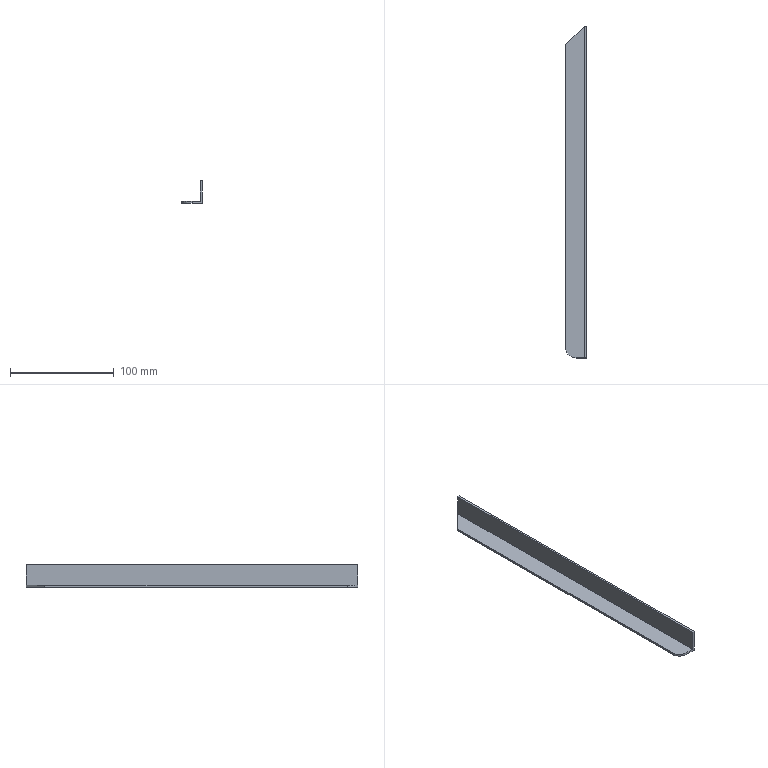Part | STEP file | Rear Closing Plate Frame Lower 4 | 1 solid | 10 faces | box 20 x 320 x 22 mm | volume 25233 mm3 | plane 9 | cylinder 1 | commonest cylinder face diameters 20 x1
STEP:
#1=CARTESIAN_POINT('',(687.249,25.392,22.));
#2=VERTEX_POINT('',#1);
#3=CARTESIAN_POINT('',(687.249,25.392,0.));
#4=VERTEX_POINT('',#3);
#5=CARTESIAN_POINT('',(687.249,25.392,22.));
#6=DIRECTION('',(0.,0.,-1.));
#7=VECTOR('',#6,1000.);
#8=LINE('',#5,#7);
#9=EDGE_CURVE('',#2,#4,#8,.T.);
#10=ORIENTED_EDGE('',*,*,#9,.F.);
#11=CARTESIAN_POINT('',(687.249,-294.608,22.));
#12=VERTEX_POINT('',#11);
#13=CARTESIAN_POINT('',(687.249,27.392,22.));
#14=DIRECTION('',(0.,1.,0.));
#15=VECTOR('',#14,1000.);
#16=LINE('',#13,#15);
#17=EDGE_CURVE('',#12,#2,#16,.T.);
#18=ORIENTED_EDGE('',*,*,#17,.F.);
#19=CARTESIAN_POINT('',(687.249,-294.608,0.));
#20=VERTEX_POINT('',#19);
#21=CARTESIAN_POINT('',(687.249,-294.608,22.));
#22=DIRECTION('',(0.,0.,1.));
#23=VECTOR('',#22,1000.);
#24=LINE('',#21,#23);
#25=EDGE_CURVE('',#20,#12,#24,.T.);
#26=ORIENTED_EDGE('',*,*,#25,.F.);
#27=CARTESIAN_POINT('',(687.249,27.392,0.));
#28=DIRECTION('',(0.,-1.,0.));
#29=VECTOR('',#28,1000.);
#30=LINE('',#27,#29);
#31=EDGE_CURVE('',#4,#20,#30,.T.);
#32=ORIENTED_EDGE('',*,*,#31,.F.);
#33=EDGE_LOOP('',(#10,#18,#26,#32));
#34=FACE_OUTER_BOUND('',#33,.T.);
#35=CARTESIAN_POINT('',(687.249,27.392,22.));
#36=DIRECTION('',(-1.,0.,0.));
#37=DIRECTION('',(0.,0.,1.));
#38=AXIS2_PLACEMENT_3D('',#35,#36,#37);
#39=PLANE('',#38);
#40=ADVANCED_FACE('',(#34),#39,.F.);
#41=CARTESIAN_POINT('',(685.249,25.392,0.));
#42=VERTEX_POINT('',#41);
#43=CARTESIAN_POINT('',(0.,25.392,0.));
#44=DIRECTION('',(1.,0.,0.));
#45=VECTOR('',#44,1000.);
#46=LINE('',#43,#45);
#47=EDGE_CURVE('',#42,#4,#46,.T.);
#48=ORIENTED_EDGE('',*,*,#47,.T.);
#49=ORIENTED_EDGE('',*,*,#31,.T.);
#50=CARTESIAN_POINT('',(677.249,-294.608,0.));
#51=VERTEX_POINT('',#50);
#52=CARTESIAN_POINT('',(0.,-294.608,0.));
#53=DIRECTION('',(-1.,0.,0.));
#54=VECTOR('',#53,1000.);
#55=LINE('',#52,#54);
#56=EDGE_CURVE('',#20,#51,#55,.T.);
#57=ORIENTED_EDGE('',*,*,#56,.T.);
#58=CARTESIAN_POINT('',(667.249,-284.608,0.));
#59=VERTEX_POINT('',#58);
#60=CARTESIAN_POINT('',(677.249,-284.608,0.));
#61=DIRECTION('',(0.,0.,-1.));
#62=DIRECTION('',(1.,0.,0.));
#63=AXIS2_PLACEMENT_3D('',#60,#61,#62);
#64=CIRCLE('',#63,10.);
#65=EDGE_CURVE('',#51,#59,#64,.T.);
#66=ORIENTED_EDGE('',*,*,#65,.T.);
#67=CARTESIAN_POINT('',(667.249,7.392,0.));
#68=VERTEX_POINT('',#67);
#69=CARTESIAN_POINT('',(667.249,0.,0.));
#70=DIRECTION('',(0.,1.,0.));
#71=VECTOR('',#70,1000.);
#72=LINE('',#69,#71);
#73=EDGE_CURVE('',#59,#68,#72,.T.);
#74=ORIENTED_EDGE('',*,*,#73,.T.);
#75=CARTESIAN_POINT('',(667.249,7.392,0.));
#76=DIRECTION('',(0.7071,0.7071,0.));
#77=VECTOR('',#76,1000.);
#78=LINE('',#75,#77);
#79=EDGE_CURVE('',#68,#42,#78,.T.);
#80=ORIENTED_EDGE('',*,*,#79,.T.);
#81=EDGE_LOOP('',(#48,#49,#57,#66,#74,#80));
#82=FACE_OUTER_BOUND('',#81,.T.);
#83=CARTESIAN_POINT('',(0.,0.,0.));
#84=DIRECTION('',(0.,0.,-1.));
#85=DIRECTION('',(-1.,0.,0.));
#86=AXIS2_PLACEMENT_3D('',#83,#84,#85);
#87=PLANE('',#86);
#88=ADVANCED_FACE('',(#82),#87,.T.);
#89=CARTESIAN_POINT('',(685.249,25.392,2.));
#90=VERTEX_POINT('',#89);
#91=CARTESIAN_POINT('',(685.249,25.392,22.));
#92=DIRECTION('',(0.,0.,-1.));
#93=VECTOR('',#92,1000.);
#94=LINE('',#91,#93);
#95=EDGE_CURVE('',#90,#42,#94,.T.);
#96=ORIENTED_EDGE('',*,*,#95,.F.);
#97=CARTESIAN_POINT('',(685.249,25.392,22.));
#98=VERTEX_POINT('',#97);
#99=CARTESIAN_POINT('',(685.249,25.392,22.));
#100=DIRECTION('',(0.,0.,-1.));
#101=VECTOR('',#100,1000.);
#102=LINE('',#99,#101);
#103=EDGE_CURVE('',#98,#90,#102,.T.);
#104=ORIENTED_EDGE('',*,*,#103,.F.);
#105=CARTESIAN_POINT('',(687.249,25.392,22.));
#106=DIRECTION('',(-1.,0.,0.));
#107=VECTOR('',#106,1000.);
#108=LINE('',#105,#107);
#109=EDGE_CURVE('',#2,#98,#108,.T.);
#110=ORIENTED_EDGE('',*,*,#109,.F.);
#111=ORIENTED_EDGE('',*,*,#9,.T.);
#112=ORIENTED_EDGE('',*,*,#47,.F.);
#113=EDGE_LOOP('',(#96,#104,#110,#111,#112));
#114=FACE_OUTER_BOUND('',#113,.T.);
#115=CARTESIAN_POINT('',(687.249,25.392,22.));
#116=DIRECTION('',(0.,-1.,0.));
#117=DIRECTION('',(1.,0.,0.));
#118=AXIS2_PLACEMENT_3D('',#115,#116,#117);
#119=PLANE('',#118);
#120=ADVANCED_FACE('',(#114),#119,.F.);
#121=ORIENTED_EDGE('',*,*,#109,.T.);
#122=CARTESIAN_POINT('',(685.249,-294.608,22.));
#123=VERTEX_POINT('',#122);
#124=CARTESIAN_POINT('',(685.249,0.,22.));
#125=DIRECTION('',(0.,1.,0.));
#126=VECTOR('',#125,1000.);
#127=LINE('',#124,#126);
#128=EDGE_CURVE('',#123,#98,#127,.T.);
#129=ORIENTED_EDGE('',*,*,#128,.F.);
#130=CARTESIAN_POINT('',(0.,-294.608,22.));
#131=DIRECTION('',(-1.,0.,0.));
#132=VECTOR('',#131,1000.);
#133=LINE('',#130,#132);
#134=EDGE_CURVE('',#12,#123,#133,.T.);
#135=ORIENTED_EDGE('',*,*,#134,.F.);
#136=ORIENTED_EDGE('',*,*,#17,.T.);
#137=EDGE_LOOP('',(#121,#129,#135,#136));
#138=FACE_OUTER_BOUND('',#137,.T.);
#139=CARTESIAN_POINT('',(0.,0.,22.));
#140=DIRECTION('',(0.,0.,-1.));
#141=DIRECTION('',(-1.,0.,0.));
#142=AXIS2_PLACEMENT_3D('',#139,#140,#141);
#143=PLANE('',#142);
#144=ADVANCED_FACE('',(#138),#143,.F.);
#145=CARTESIAN_POINT('',(677.249,-294.608,2.));
#146=VERTEX_POINT('',#145);
#147=CARTESIAN_POINT('',(677.249,-294.608,22.));
#148=DIRECTION('',(0.,0.,1.));
#149=VECTOR('',#148,1000.);
#150=LINE('',#147,#149);
#151=EDGE_CURVE('',#51,#146,#150,.T.);
#152=ORIENTED_EDGE('',*,*,#151,.F.);
#153=ORIENTED_EDGE('',*,*,#56,.F.);
#154=ORIENTED_EDGE('',*,*,#25,.T.);
#155=ORIENTED_EDGE('',*,*,#134,.T.);
#156=CARTESIAN_POINT('',(685.249,-294.608,2.));
#157=VERTEX_POINT('',#156);
#158=CARTESIAN_POINT('',(685.249,-294.608,22.));
#159=DIRECTION('',(0.,0.,1.));
#160=VECTOR('',#159,1000.);
#161=LINE('',#158,#160);
#162=EDGE_CURVE('',#157,#123,#161,.T.);
#163=ORIENTED_EDGE('',*,*,#162,.F.);
#164=CARTESIAN_POINT('',(-3.251,-294.608,2.));
#165=DIRECTION('',(1.,0.,0.));
#166=VECTOR('',#165,1000.);
#167=LINE('',#164,#166);
#168=EDGE_CURVE('',#146,#157,#167,.T.);
#169=ORIENTED_EDGE('',*,*,#168,.F.);
#170=EDGE_LOOP('',(#152,#153,#154,#155,#163,#169));
#171=FACE_OUTER_BOUND('',#170,.T.);
#172=CARTESIAN_POINT('',(-3.251,-294.608,22.));
#173=DIRECTION('',(0.,1.,0.));
#174=DIRECTION('',(-1.,0.,0.));
#175=AXIS2_PLACEMENT_3D('',#172,#173,#174);
#176=PLANE('',#175);
#177=ADVANCED_FACE('',(#171),#176,.F.);
#178=ORIENTED_EDGE('',*,*,#79,.F.);
#179=CARTESIAN_POINT('',(667.249,7.392,2.));
#180=VERTEX_POINT('',#179);
#181=CARTESIAN_POINT('',(667.249,7.392,22.));
#182=DIRECTION('',(0.,0.,-1.));
#183=VECTOR('',#182,1000.);
#184=LINE('',#181,#183);
#185=EDGE_CURVE('',#180,#68,#184,.T.);
#186=ORIENTED_EDGE('',*,*,#185,.F.);
#187=CARTESIAN_POINT('',(667.249,7.392,2.));
#188=DIRECTION('',(-0.7071,-0.7071,0.));
#189=VECTOR('',#188,1000.);
#190=LINE('',#187,#189);
#191=EDGE_CURVE('',#90,#180,#190,.T.);
#192=ORIENTED_EDGE('',*,*,#191,.F.);
#193=ORIENTED_EDGE('',*,*,#95,.T.);
#194=EDGE_LOOP('',(#178,#186,#192,#193));
#195=FACE_OUTER_BOUND('',#194,.T.);
#196=CARTESIAN_POINT('',(667.249,7.392,22.));
#197=DIRECTION('',(0.7071,-0.7071,0.));
#198=DIRECTION('',(0.7071,0.7071,0.));
#199=AXIS2_PLACEMENT_3D('',#196,#197,#198);
#200=PLANE('',#199);
#201=ADVANCED_FACE('',(#195),#200,.F.);
#202=CARTESIAN_POINT('',(667.249,-284.608,2.));
#203=VERTEX_POINT('',#202);
#204=CARTESIAN_POINT('',(667.249,7.392,2.));
#205=DIRECTION('',(0.,1.,0.));
#206=VECTOR('',#205,1000.);
#207=LINE('',#204,#206);
#208=EDGE_CURVE('',#203,#180,#207,.T.);
#209=ORIENTED_EDGE('',*,*,#208,.T.);
#210=ORIENTED_EDGE('',*,*,#185,.T.);
#211=ORIENTED_EDGE('',*,*,#73,.F.);
#212=CARTESIAN_POINT('',(667.249,-284.608,22.));
#213=DIRECTION('',(0.,0.,1.));
#214=VECTOR('',#213,1000.);
#215=LINE('',#212,#214);
#216=EDGE_CURVE('',#59,#203,#215,.T.);
#217=ORIENTED_EDGE('',*,*,#216,.T.);
#218=EDGE_LOOP('',(#209,#210,#211,#217));
#219=FACE_OUTER_BOUND('',#218,.T.);
#220=CARTESIAN_POINT('',(667.249,7.392,22.));
#221=DIRECTION('',(-1.,0.,0.));
#222=DIRECTION('',(0.,0.,1.));
#223=AXIS2_PLACEMENT_3D('',#220,#221,#222);
#224=PLANE('',#223);
#225=ADVANCED_FACE('',(#219),#224,.T.);
#226=ORIENTED_EDGE('',*,*,#65,.F.);
#227=ORIENTED_EDGE('',*,*,#151,.T.);
#228=CARTESIAN_POINT('',(677.249,-284.608,2.));
#229=DIRECTION('',(0.,0.,-1.));
#230=DIRECTION('',(1.,0.,0.));
#231=AXIS2_PLACEMENT_3D('',#228,#229,#230);
#232=CIRCLE('',#231,10.);
#233=EDGE_CURVE('',#146,#203,#232,.T.);
#234=ORIENTED_EDGE('',*,*,#233,.T.);
#235=ORIENTED_EDGE('',*,*,#216,.F.);
#236=EDGE_LOOP('',(#226,#227,#234,#235));
#237=FACE_OUTER_BOUND('',#236,.T.);
#238=CARTESIAN_POINT('',(677.249,-284.608,22.));
#239=DIRECTION('',(0.,0.,1.));
#240=DIRECTION('',(1.,0.,0.));
#241=AXIS2_PLACEMENT_3D('',#238,#239,#240);
#242=CYLINDRICAL_SURFACE('',#241,10.);
#243=ADVANCED_FACE('',(#237),#242,.T.);
#244=ORIENTED_EDGE('',*,*,#128,.T.);
#245=ORIENTED_EDGE('',*,*,#103,.T.);
#246=CARTESIAN_POINT('',(685.249,27.392,2.));
#247=DIRECTION('',(0.,-1.,0.));
#248=VECTOR('',#247,1000.);
#249=LINE('',#246,#248);
#250=EDGE_CURVE('',#90,#157,#249,.T.);
#251=ORIENTED_EDGE('',*,*,#250,.T.);
#252=ORIENTED_EDGE('',*,*,#162,.T.);
#253=EDGE_LOOP('',(#244,#245,#251,#252));
#254=FACE_OUTER_BOUND('',#253,.T.);
#255=CARTESIAN_POINT('',(685.249,27.392,22.));
#256=DIRECTION('',(-1.,0.,0.));
#257=DIRECTION('',(0.,0.,1.));
#258=AXIS2_PLACEMENT_3D('',#255,#256,#257);
#259=PLANE('',#258);
#260=ADVANCED_FACE('',(#254),#259,.T.);
#261=ORIENTED_EDGE('',*,*,#233,.F.);
#262=ORIENTED_EDGE('',*,*,#168,.T.);
#263=ORIENTED_EDGE('',*,*,#250,.F.);
#264=ORIENTED_EDGE('',*,*,#191,.T.);
#265=ORIENTED_EDGE('',*,*,#208,.F.);
#266=EDGE_LOOP('',(#261,#262,#263,#264,#265));
#267=FACE_OUTER_BOUND('',#266,.T.);
#268=CARTESIAN_POINT('',(0.,0.,2.));
#269=DIRECTION('',(0.,0.,-1.));
#270=DIRECTION('',(-1.,0.,0.));
#271=AXIS2_PLACEMENT_3D('',#268,#269,#270);
#272=PLANE('',#271);
#273=ADVANCED_FACE('',(#267),#272,.F.);
#274=CLOSED_SHELL('',(#40,#88,#120,#144,#177,#201,#225,#243,#260,#273));
#275=MANIFOLD_SOLID_BREP('',#274);
#276=CARTESIAN_POINT('',(0.,0.,0.));
#277=DIRECTION('',(0.,0.,1.));
#278=DIRECTION('',(1.,0.,0.));
#279=AXIS2_PLACEMENT_3D('',#276,#277,#278);
#280=(LENGTH_UNIT()NAMED_UNIT(*)SI_UNIT(.MILLI.,.METRE.));
#281=UNCERTAINTY_MEASURE_WITH_UNIT(LENGTH_MEASURE(0.00001),#280,'','');
#282=(NAMED_UNIT(*)PLANE_ANGLE_UNIT()SI_UNIT($,.RADIAN.));
#283=(NAMED_UNIT(*)SI_UNIT($,.STERADIAN.)SOLID_ANGLE_UNIT());
#284=(GEOMETRIC_REPRESENTATION_CONTEXT(3)GLOBAL_UNCERTAINTY_ASSIGNED_CONTEXT((#281))GLOBAL_UNIT_ASSIGNED_CONTEXT((#280,#282,#283))REPRESENTATION_CONTEXT('',''));
#285=ADVANCED_BREP_SHAPE_REPRESENTATION('',(#275,#279),#284);